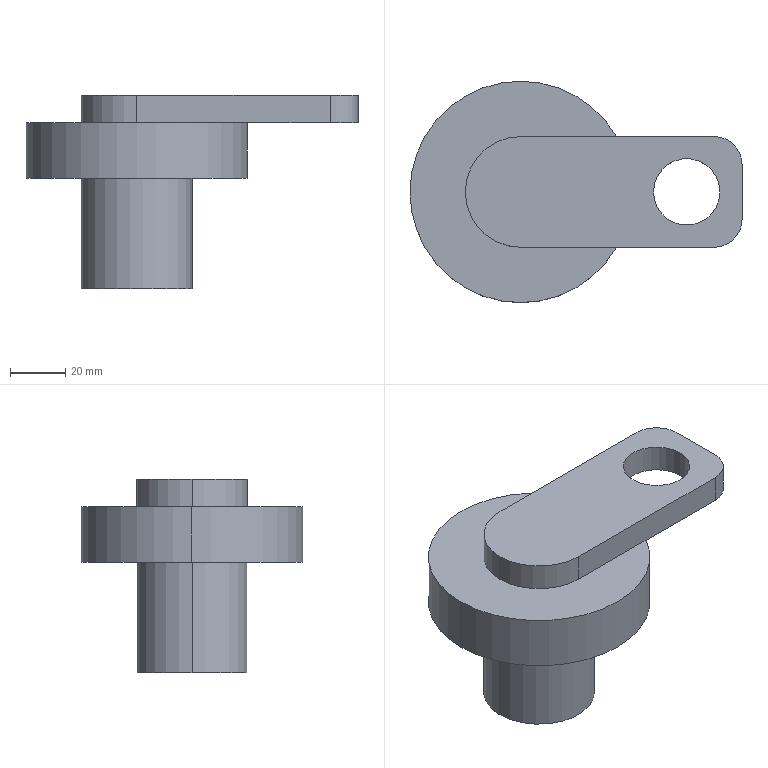Part | SolidWorks | features ICE 4, Extrusion 1, Fillet 1 | 1 solid | 18 faces | box 120 x 80 x 70 mm | volume 184127 mm3 | cylinder 10 | plane 8 | commonest cylinder face diameters 40 x4 20 x2 24 x2 80 x2
STEP:
#1=CARTESIAN_POINT('',(-10.,0.,-20.));
#2=VERTEX_POINT('',#1);
#3=CARTESIAN_POINT('',(-50.,0.,-20.));
#4=VERTEX_POINT('',#3);
#5=CARTESIAN_POINT('',(-30.,0.,-20.));
#6=DIRECTION('',(0.,0.,1.));
#7=DIRECTION('',(-1.,0.,0.));
#8=AXIS2_PLACEMENT_3D('',#5,#6,#7);
#9=CIRCLE('',#8,20.);
#10=EDGE_CURVE('',#2,#4,#9,.T.);
#11=ORIENTED_EDGE('',*,*,#10,.F.);
#12=CARTESIAN_POINT('',(-10.,0.,-60.));
#13=VERTEX_POINT('',#12);
#14=CARTESIAN_POINT('',(-10.,0.,10.));
#15=DIRECTION('',(0.,0.,-1.));
#16=VECTOR('',#15,1000.);
#17=LINE('',#14,#16);
#18=EDGE_CURVE('',#2,#13,#17,.T.);
#19=ORIENTED_EDGE('',*,*,#18,.T.);
#20=CARTESIAN_POINT('',(-50.,0.,-60.));
#21=VERTEX_POINT('',#20);
#22=CARTESIAN_POINT('',(-30.,0.,-60.));
#23=DIRECTION('',(0.,0.,-1.));
#24=DIRECTION('',(-1.,0.,0.));
#25=AXIS2_PLACEMENT_3D('',#22,#23,#24);
#26=CIRCLE('',#25,20.);
#27=EDGE_CURVE('',#21,#13,#26,.T.);
#28=ORIENTED_EDGE('',*,*,#27,.F.);
#29=CARTESIAN_POINT('',(-50.,0.,10.));
#30=DIRECTION('',(0.,0.,-1.));
#31=VECTOR('',#30,1000.);
#32=LINE('',#29,#31);
#33=EDGE_CURVE('',#4,#21,#32,.T.);
#34=ORIENTED_EDGE('',*,*,#33,.F.);
#35=EDGE_LOOP('',(#11,#19,#28,#34));
#36=FACE_OUTER_BOUND('',#35,.T.);
#37=CARTESIAN_POINT('',(-30.,0.,10.));
#38=DIRECTION('',(0.,0.,-1.));
#39=DIRECTION('',(-1.,0.,0.));
#40=AXIS2_PLACEMENT_3D('',#37,#38,#39);
#41=CYLINDRICAL_SURFACE('',#40,20.);
#42=ADVANCED_FACE('',(#36),#41,.T.);
#43=CARTESIAN_POINT('',(-70.,0.,-20.));
#44=VERTEX_POINT('',#43);
#45=CARTESIAN_POINT('',(10.,0.,-20.));
#46=VERTEX_POINT('',#45);
#47=CARTESIAN_POINT('',(-30.,0.,-20.));
#48=DIRECTION('',(0.,0.,-1.));
#49=DIRECTION('',(-1.,0.,0.));
#50=AXIS2_PLACEMENT_3D('',#47,#48,#49);
#51=CIRCLE('',#50,40.);
#52=EDGE_CURVE('',#44,#46,#51,.T.);
#53=ORIENTED_EDGE('',*,*,#52,.F.);
#54=CARTESIAN_POINT('',(-70.,0.,0.));
#55=VERTEX_POINT('',#54);
#56=CARTESIAN_POINT('',(-70.,0.,-20.));
#57=DIRECTION('',(0.,0.,1.));
#58=VECTOR('',#57,1000.);
#59=LINE('',#56,#58);
#60=EDGE_CURVE('',#44,#55,#59,.T.);
#61=ORIENTED_EDGE('',*,*,#60,.T.);
#62=CARTESIAN_POINT('',(4.641,20.,0.));
#63=VERTEX_POINT('',#62);
#64=CARTESIAN_POINT('',(-30.,0.,0.));
#65=DIRECTION('',(0.,0.,-1.));
#66=DIRECTION('',(-1.,0.,0.));
#67=AXIS2_PLACEMENT_3D('',#64,#65,#66);
#68=CIRCLE('',#67,40.);
#69=EDGE_CURVE('',#55,#63,#68,.T.);
#70=ORIENTED_EDGE('',*,*,#69,.T.);
#71=CARTESIAN_POINT('',(10.,0.,0.));
#72=VERTEX_POINT('',#71);
#73=CARTESIAN_POINT('',(-30.,0.,0.));
#74=DIRECTION('',(0.,0.,-1.));
#75=DIRECTION('',(-1.,0.,0.));
#76=AXIS2_PLACEMENT_3D('',#73,#74,#75);
#77=CIRCLE('',#76,40.);
#78=EDGE_CURVE('',#63,#72,#77,.T.);
#79=ORIENTED_EDGE('',*,*,#78,.T.);
#80=CARTESIAN_POINT('',(10.,0.,-20.));
#81=DIRECTION('',(0.,0.,1.));
#82=VECTOR('',#81,1000.);
#83=LINE('',#80,#82);
#84=EDGE_CURVE('',#46,#72,#83,.T.);
#85=ORIENTED_EDGE('',*,*,#84,.F.);
#86=EDGE_LOOP('',(#53,#61,#70,#79,#85));
#87=FACE_OUTER_BOUND('',#86,.T.);
#88=CARTESIAN_POINT('',(-30.,0.,-20.));
#89=DIRECTION('',(0.,0.,1.));
#90=DIRECTION('',(1.,0.,0.));
#91=AXIS2_PLACEMENT_3D('',#88,#89,#90);
#92=CYLINDRICAL_SURFACE('',#91,40.);
#93=ADVANCED_FACE('',(#87),#92,.T.);
#94=CARTESIAN_POINT('',(18.,0.,0.));
#95=VERTEX_POINT('',#94);
#96=CARTESIAN_POINT('',(42.,0.,0.));
#97=VERTEX_POINT('',#96);
#98=CARTESIAN_POINT('',(30.,0.,0.));
#99=DIRECTION('',(0.,0.,1.));
#100=DIRECTION('',(1.,0.,0.));
#101=AXIS2_PLACEMENT_3D('',#98,#99,#100);
#102=CIRCLE('',#101,12.);
#103=EDGE_CURVE('',#95,#97,#102,.T.);
#104=ORIENTED_EDGE('',*,*,#103,.F.);
#105=CARTESIAN_POINT('',(18.,0.,10.));
#106=VERTEX_POINT('',#105);
#107=CARTESIAN_POINT('',(18.,0.,0.));
#108=DIRECTION('',(0.,0.,1.));
#109=VECTOR('',#108,1000.);
#110=LINE('',#107,#109);
#111=EDGE_CURVE('',#95,#106,#110,.T.);
#112=ORIENTED_EDGE('',*,*,#111,.T.);
#113=CARTESIAN_POINT('',(42.,0.,10.));
#114=VERTEX_POINT('',#113);
#115=CARTESIAN_POINT('',(30.,0.,10.));
#116=DIRECTION('',(0.,0.,1.));
#117=DIRECTION('',(1.,0.,0.));
#118=AXIS2_PLACEMENT_3D('',#115,#116,#117);
#119=CIRCLE('',#118,12.);
#120=EDGE_CURVE('',#106,#114,#119,.T.);
#121=ORIENTED_EDGE('',*,*,#120,.T.);
#122=CARTESIAN_POINT('',(42.,0.,0.));
#123=DIRECTION('',(0.,0.,1.));
#124=VECTOR('',#123,1000.);
#125=LINE('',#122,#124);
#126=EDGE_CURVE('',#97,#114,#125,.T.);
#127=ORIENTED_EDGE('',*,*,#126,.F.);
#128=EDGE_LOOP('',(#104,#112,#121,#127));
#129=FACE_OUTER_BOUND('',#128,.T.);
#130=CARTESIAN_POINT('',(30.,0.,0.));
#131=DIRECTION('',(0.,0.,1.));
#132=DIRECTION('',(1.,0.,0.));
#133=AXIS2_PLACEMENT_3D('',#130,#131,#132);
#134=CYLINDRICAL_SURFACE('',#133,12.);
#135=ADVANCED_FACE('',(#129),#134,.F.);
#136=CARTESIAN_POINT('',(-30.,-20.,10.));
#137=VERTEX_POINT('',#136);
#138=CARTESIAN_POINT('',(-50.,0.,10.));
#139=VERTEX_POINT('',#138);
#140=CARTESIAN_POINT('',(-30.,0.,10.));
#141=DIRECTION('',(0.,0.,-1.));
#142=DIRECTION('',(-1.,0.,0.));
#143=AXIS2_PLACEMENT_3D('',#140,#141,#142);
#144=CIRCLE('',#143,20.);
#145=EDGE_CURVE('',#137,#139,#144,.T.);
#146=ORIENTED_EDGE('',*,*,#145,.T.);
#147=CARTESIAN_POINT('',(-50.,0.,0.));
#148=VERTEX_POINT('',#147);
#149=CARTESIAN_POINT('',(-50.,0.,10.));
#150=DIRECTION('',(0.,0.,-1.));
#151=VECTOR('',#150,1000.);
#152=LINE('',#149,#151);
#153=EDGE_CURVE('',#139,#148,#152,.T.);
#154=ORIENTED_EDGE('',*,*,#153,.T.);
#155=CARTESIAN_POINT('',(-30.,-20.,0.));
#156=VERTEX_POINT('',#155);
#157=CARTESIAN_POINT('',(-30.,0.,0.));
#158=DIRECTION('',(0.,0.,1.));
#159=DIRECTION('',(-1.,0.,0.));
#160=AXIS2_PLACEMENT_3D('',#157,#158,#159);
#161=CIRCLE('',#160,20.);
#162=EDGE_CURVE('',#148,#156,#161,.T.);
#163=ORIENTED_EDGE('',*,*,#162,.T.);
#164=CARTESIAN_POINT('',(-30.,-20.,10.));
#165=DIRECTION('',(0.,0.,-1.));
#166=VECTOR('',#165,1000.);
#167=LINE('',#164,#166);
#168=EDGE_CURVE('',#137,#156,#167,.T.);
#169=ORIENTED_EDGE('',*,*,#168,.F.);
#170=EDGE_LOOP('',(#146,#154,#163,#169));
#171=FACE_OUTER_BOUND('',#170,.T.);
#172=CARTESIAN_POINT('',(-30.,0.,10.));
#173=DIRECTION('',(0.,0.,-1.));
#174=DIRECTION('',(-1.,0.,0.));
#175=AXIS2_PLACEMENT_3D('',#172,#173,#174);
#176=CYLINDRICAL_SURFACE('',#175,20.);
#177=ADVANCED_FACE('',(#171),#176,.T.);
#178=ORIENTED_EDGE('',*,*,#153,.F.);
#179=CARTESIAN_POINT('',(-30.,20.,10.));
#180=VERTEX_POINT('',#179);
#181=CARTESIAN_POINT('',(-30.,0.,10.));
#182=DIRECTION('',(0.,0.,-1.));
#183=DIRECTION('',(-1.,0.,0.));
#184=AXIS2_PLACEMENT_3D('',#181,#182,#183);
#185=CIRCLE('',#184,20.);
#186=EDGE_CURVE('',#139,#180,#185,.T.);
#187=ORIENTED_EDGE('',*,*,#186,.T.);
#188=CARTESIAN_POINT('',(-30.,20.,0.));
#189=VERTEX_POINT('',#188);
#190=CARTESIAN_POINT('',(-30.,20.,10.));
#191=DIRECTION('',(0.,0.,-1.));
#192=VECTOR('',#191,1000.);
#193=LINE('',#190,#192);
#194=EDGE_CURVE('',#180,#189,#193,.T.);
#195=ORIENTED_EDGE('',*,*,#194,.T.);
#196=CARTESIAN_POINT('',(-30.,0.,0.));
#197=DIRECTION('',(0.,0.,1.));
#198=DIRECTION('',(-1.,0.,0.));
#199=AXIS2_PLACEMENT_3D('',#196,#197,#198);
#200=CIRCLE('',#199,20.);
#201=EDGE_CURVE('',#189,#148,#200,.T.);
#202=ORIENTED_EDGE('',*,*,#201,.T.);
#203=EDGE_LOOP('',(#178,#187,#195,#202));
#204=FACE_OUTER_BOUND('',#203,.T.);
#205=CARTESIAN_POINT('',(-30.,0.,10.));
#206=DIRECTION('',(0.,0.,-1.));
#207=DIRECTION('',(-1.,0.,0.));
#208=AXIS2_PLACEMENT_3D('',#205,#206,#207);
#209=CYLINDRICAL_SURFACE('',#208,20.);
#210=ADVANCED_FACE('',(#204),#209,.T.);
#211=ORIENTED_EDGE('',*,*,#78,.F.);
#212=CARTESIAN_POINT('',(40.,20.,0.));
#213=VERTEX_POINT('',#212);
#214=CARTESIAN_POINT('',(-50.,20.,0.));
#215=DIRECTION('',(-1.,0.,0.));
#216=VECTOR('',#215,1000.);
#217=LINE('',#214,#216);
#218=EDGE_CURVE('',#213,#63,#217,.T.);
#219=ORIENTED_EDGE('',*,*,#218,.F.);
#220=CARTESIAN_POINT('',(50.,10.,0.));
#221=VERTEX_POINT('',#220);
#222=CARTESIAN_POINT('',(40.,10.,0.));
#223=DIRECTION('',(0.,0.,-1.));
#224=DIRECTION('',(1.,0.,0.));
#225=AXIS2_PLACEMENT_3D('',#222,#223,#224);
#226=CIRCLE('',#225,10.);
#227=EDGE_CURVE('',#213,#221,#226,.T.);
#228=ORIENTED_EDGE('',*,*,#227,.T.);
#229=CARTESIAN_POINT('',(50.,-10.,0.));
#230=VERTEX_POINT('',#229);
#231=CARTESIAN_POINT('',(50.,20.,0.));
#232=DIRECTION('',(0.,1.,0.));
#233=VECTOR('',#232,1000.);
#234=LINE('',#231,#233);
#235=EDGE_CURVE('',#230,#221,#234,.T.);
#236=ORIENTED_EDGE('',*,*,#235,.F.);
#237=CARTESIAN_POINT('',(40.,-20.,0.));
#238=VERTEX_POINT('',#237);
#239=CARTESIAN_POINT('',(40.,-10.,0.));
#240=DIRECTION('',(0.,0.,-1.));
#241=DIRECTION('',(1.,0.,0.));
#242=AXIS2_PLACEMENT_3D('',#239,#240,#241);
#243=CIRCLE('',#242,10.);
#244=EDGE_CURVE('',#230,#238,#243,.T.);
#245=ORIENTED_EDGE('',*,*,#244,.T.);
#246=CARTESIAN_POINT('',(4.641,-20.,0.));
#247=VERTEX_POINT('',#246);
#248=CARTESIAN_POINT('',(-50.,-20.,0.));
#249=DIRECTION('',(1.,0.,0.));
#250=VECTOR('',#249,1000.);
#251=LINE('',#248,#250);
#252=EDGE_CURVE('',#247,#238,#251,.T.);
#253=ORIENTED_EDGE('',*,*,#252,.F.);
#254=CARTESIAN_POINT('',(-30.,0.,0.));
#255=DIRECTION('',(0.,0.,-1.));
#256=DIRECTION('',(-1.,0.,0.));
#257=AXIS2_PLACEMENT_3D('',#254,#255,#256);
#258=CIRCLE('',#257,40.);
#259=EDGE_CURVE('',#72,#247,#258,.T.);
#260=ORIENTED_EDGE('',*,*,#259,.F.);
#261=EDGE_LOOP('',(#211,#219,#228,#236,#245,#253,#260));
#262=FACE_OUTER_BOUND('',#261,.T.);
#263=CARTESIAN_POINT('',(30.,0.,0.));
#264=DIRECTION('',(0.,0.,1.));
#265=DIRECTION('',(1.,0.,0.));
#266=AXIS2_PLACEMENT_3D('',#263,#264,#265);
#267=CIRCLE('',#266,12.);
#268=EDGE_CURVE('',#97,#95,#267,.T.);
#269=ORIENTED_EDGE('',*,*,#268,.T.);
#270=ORIENTED_EDGE('',*,*,#103,.T.);
#271=EDGE_LOOP('',(#269,#270));
#272=FACE_BOUND('',#271,.T.);
#273=CARTESIAN_POINT('',(0.,0.,0.));
#274=DIRECTION('',(0.,0.,1.));
#275=DIRECTION('',(1.,0.,0.));
#276=AXIS2_PLACEMENT_3D('',#273,#274,#275);
#277=PLANE('',#276);
#278=ADVANCED_FACE('',(#262,#272),#277,.F.);
#279=CARTESIAN_POINT('',(30.,0.,10.));
#280=DIRECTION('',(0.,0.,1.));
#281=DIRECTION('',(1.,0.,0.));
#282=AXIS2_PLACEMENT_3D('',#279,#280,#281);
#283=CIRCLE('',#282,12.);
#284=EDGE_CURVE('',#114,#106,#283,.T.);
#285=ORIENTED_EDGE('',*,*,#284,.F.);
#286=ORIENTED_EDGE('',*,*,#120,.F.);
#287=EDGE_LOOP('',(#285,#286));
#288=FACE_BOUND('',#287,.T.);
#289=ORIENTED_EDGE('',*,*,#145,.F.);
#290=CARTESIAN_POINT('',(40.,-20.,10.));
#291=VERTEX_POINT('',#290);
#292=CARTESIAN_POINT('',(-50.,-20.,10.));
#293=DIRECTION('',(1.,0.,0.));
#294=VECTOR('',#293,1000.);
#295=LINE('',#292,#294);
#296=EDGE_CURVE('',#137,#291,#295,.T.);
#297=ORIENTED_EDGE('',*,*,#296,.T.);
#298=CARTESIAN_POINT('',(50.,-10.,10.));
#299=VERTEX_POINT('',#298);
#300=CARTESIAN_POINT('',(40.,-10.,10.));
#301=DIRECTION('',(0.,0.,1.));
#302=DIRECTION('',(1.,0.,0.));
#303=AXIS2_PLACEMENT_3D('',#300,#301,#302);
#304=CIRCLE('',#303,10.);
#305=EDGE_CURVE('',#291,#299,#304,.T.);
#306=ORIENTED_EDGE('',*,*,#305,.T.);
#307=CARTESIAN_POINT('',(50.,10.,10.));
#308=VERTEX_POINT('',#307);
#309=CARTESIAN_POINT('',(50.,20.,10.));
#310=DIRECTION('',(0.,1.,0.));
#311=VECTOR('',#310,1000.);
#312=LINE('',#309,#311);
#313=EDGE_CURVE('',#299,#308,#312,.T.);
#314=ORIENTED_EDGE('',*,*,#313,.T.);
#315=CARTESIAN_POINT('',(40.,20.,10.));
#316=VERTEX_POINT('',#315);
#317=CARTESIAN_POINT('',(40.,10.,10.));
#318=DIRECTION('',(0.,0.,1.));
#319=DIRECTION('',(1.,0.,0.));
#320=AXIS2_PLACEMENT_3D('',#317,#318,#319);
#321=CIRCLE('',#320,10.);
#322=EDGE_CURVE('',#308,#316,#321,.T.);
#323=ORIENTED_EDGE('',*,*,#322,.T.);
#324=CARTESIAN_POINT('',(-50.,20.,10.));
#325=DIRECTION('',(-1.,0.,0.));
#326=VECTOR('',#325,1000.);
#327=LINE('',#324,#326);
#328=EDGE_CURVE('',#316,#180,#327,.T.);
#329=ORIENTED_EDGE('',*,*,#328,.T.);
#330=ORIENTED_EDGE('',*,*,#186,.F.);
#331=EDGE_LOOP('',(#289,#297,#306,#314,#323,#329,#330));
#332=FACE_OUTER_BOUND('',#331,.T.);
#333=CARTESIAN_POINT('',(0.,0.,10.));
#334=DIRECTION('',(0.,0.,1.));
#335=DIRECTION('',(1.,0.,0.));
#336=AXIS2_PLACEMENT_3D('',#333,#334,#335);
#337=PLANE('',#336);
#338=ADVANCED_FACE('',(#288,#332),#337,.T.);
#339=ORIENTED_EDGE('',*,*,#194,.F.);
#340=ORIENTED_EDGE('',*,*,#328,.F.);
#341=CARTESIAN_POINT('',(40.,20.,10.));
#342=DIRECTION('',(0.,0.,-1.));
#343=VECTOR('',#342,1000.);
#344=LINE('',#341,#343);
#345=EDGE_CURVE('',#316,#213,#344,.T.);
#346=ORIENTED_EDGE('',*,*,#345,.T.);
#347=ORIENTED_EDGE('',*,*,#218,.T.);
#348=CARTESIAN_POINT('',(-50.,20.,0.));
#349=DIRECTION('',(1.,0.,0.));
#350=VECTOR('',#349,1000.);
#351=LINE('',#348,#350);
#352=EDGE_CURVE('',#189,#63,#351,.T.);
#353=ORIENTED_EDGE('',*,*,#352,.F.);
#354=EDGE_LOOP('',(#339,#340,#346,#347,#353));
#355=FACE_OUTER_BOUND('',#354,.T.);
#356=CARTESIAN_POINT('',(-50.,20.,10.));
#357=DIRECTION('',(0.,-1.,0.));
#358=DIRECTION('',(0.,0.,-1.));
#359=AXIS2_PLACEMENT_3D('',#356,#357,#358);
#360=PLANE('',#359);
#361=ADVANCED_FACE('',(#355),#360,.F.);
#362=ORIENTED_EDGE('',*,*,#313,.F.);
#363=CARTESIAN_POINT('',(50.,-10.,10.));
#364=DIRECTION('',(0.,0.,-1.));
#365=VECTOR('',#364,1000.);
#366=LINE('',#363,#365);
#367=EDGE_CURVE('',#299,#230,#366,.T.);
#368=ORIENTED_EDGE('',*,*,#367,.T.);
#369=ORIENTED_EDGE('',*,*,#235,.T.);
#370=CARTESIAN_POINT('',(50.,10.,10.));
#371=DIRECTION('',(0.,0.,1.));
#372=VECTOR('',#371,1000.);
#373=LINE('',#370,#372);
#374=EDGE_CURVE('',#221,#308,#373,.T.);
#375=ORIENTED_EDGE('',*,*,#374,.T.);
#376=EDGE_LOOP('',(#362,#368,#369,#375));
#377=FACE_OUTER_BOUND('',#376,.T.);
#378=CARTESIAN_POINT('',(50.,20.,10.));
#379=DIRECTION('',(-1.,0.,0.));
#380=DIRECTION('',(0.,-1.,0.));
#381=AXIS2_PLACEMENT_3D('',#378,#379,#380);
#382=PLANE('',#381);
#383=ADVANCED_FACE('',(#377),#382,.F.);
#384=ORIENTED_EDGE('',*,*,#296,.F.);
#385=ORIENTED_EDGE('',*,*,#168,.T.);
#386=CARTESIAN_POINT('',(-50.,-20.,0.));
#387=DIRECTION('',(1.,0.,0.));
#388=VECTOR('',#387,1000.);
#389=LINE('',#386,#388);
#390=EDGE_CURVE('',#156,#247,#389,.T.);
#391=ORIENTED_EDGE('',*,*,#390,.T.);
#392=ORIENTED_EDGE('',*,*,#252,.T.);
#393=CARTESIAN_POINT('',(40.,-20.,10.));
#394=DIRECTION('',(0.,0.,1.));
#395=VECTOR('',#394,1000.);
#396=LINE('',#393,#395);
#397=EDGE_CURVE('',#238,#291,#396,.T.);
#398=ORIENTED_EDGE('',*,*,#397,.T.);
#399=EDGE_LOOP('',(#384,#385,#391,#392,#398));
#400=FACE_OUTER_BOUND('',#399,.T.);
#401=CARTESIAN_POINT('',(-50.,-20.,10.));
#402=DIRECTION('',(0.,1.,0.));
#403=DIRECTION('',(0.,0.,1.));
#404=AXIS2_PLACEMENT_3D('',#401,#402,#403);
#405=PLANE('',#404);
#406=ADVANCED_FACE('',(#400),#405,.F.);
#407=ORIENTED_EDGE('',*,*,#111,.F.);
#408=ORIENTED_EDGE('',*,*,#268,.F.);
#409=ORIENTED_EDGE('',*,*,#126,.T.);
#410=ORIENTED_EDGE('',*,*,#284,.T.);
#411=EDGE_LOOP('',(#407,#408,#409,#410));
#412=FACE_OUTER_BOUND('',#411,.T.);
#413=CARTESIAN_POINT('',(30.,0.,0.));
#414=DIRECTION('',(0.,0.,1.));
#415=DIRECTION('',(1.,0.,0.));
#416=AXIS2_PLACEMENT_3D('',#413,#414,#415);
#417=CYLINDRICAL_SURFACE('',#416,12.);
#418=ADVANCED_FACE('',(#412),#417,.F.);
#419=ORIENTED_EDGE('',*,*,#305,.F.);
#420=ORIENTED_EDGE('',*,*,#397,.F.);
#421=ORIENTED_EDGE('',*,*,#244,.F.);
#422=ORIENTED_EDGE('',*,*,#367,.F.);
#423=EDGE_LOOP('',(#419,#420,#421,#422));
#424=FACE_OUTER_BOUND('',#423,.T.);
#425=CARTESIAN_POINT('',(40.,-10.,10.));
#426=DIRECTION('',(0.,0.,-1.));
#427=DIRECTION('',(-1.,0.,0.));
#428=AXIS2_PLACEMENT_3D('',#425,#426,#427);
#429=CYLINDRICAL_SURFACE('',#428,10.);
#430=ADVANCED_FACE('',(#424),#429,.T.);
#431=ORIENTED_EDGE('',*,*,#322,.F.);
#432=ORIENTED_EDGE('',*,*,#374,.F.);
#433=ORIENTED_EDGE('',*,*,#227,.F.);
#434=ORIENTED_EDGE('',*,*,#345,.F.);
#435=EDGE_LOOP('',(#431,#432,#433,#434));
#436=FACE_OUTER_BOUND('',#435,.T.);
#437=CARTESIAN_POINT('',(40.,10.,10.));
#438=DIRECTION('',(0.,0.,-1.));
#439=DIRECTION('',(-1.,0.,0.));
#440=AXIS2_PLACEMENT_3D('',#437,#438,#439);
#441=CYLINDRICAL_SURFACE('',#440,10.);
#442=ADVANCED_FACE('',(#436),#441,.T.);
#443=ORIENTED_EDGE('',*,*,#201,.F.);
#444=ORIENTED_EDGE('',*,*,#352,.T.);
#445=ORIENTED_EDGE('',*,*,#69,.F.);
#446=CARTESIAN_POINT('',(-30.,0.,0.));
#447=DIRECTION('',(0.,0.,-1.));
#448=DIRECTION('',(-1.,0.,0.));
#449=AXIS2_PLACEMENT_3D('',#446,#447,#448);
#450=CIRCLE('',#449,40.);
#451=EDGE_CURVE('',#247,#55,#450,.T.);
#452=ORIENTED_EDGE('',*,*,#451,.F.);
#453=ORIENTED_EDGE('',*,*,#390,.F.);
#454=ORIENTED_EDGE('',*,*,#162,.F.);
#455=EDGE_LOOP('',(#443,#444,#445,#452,#453,#454));
#456=FACE_OUTER_BOUND('',#455,.T.);
#457=CARTESIAN_POINT('',(-30.,0.,0.));
#458=DIRECTION('',(0.,0.,-1.));
#459=DIRECTION('',(-1.,0.,0.));
#460=AXIS2_PLACEMENT_3D('',#457,#458,#459);
#461=PLANE('',#460);
#462=ADVANCED_FACE('',(#456),#461,.F.);
#463=ORIENTED_EDGE('',*,*,#60,.F.);
#464=CARTESIAN_POINT('',(-30.,0.,-20.));
#465=DIRECTION('',(0.,0.,-1.));
#466=DIRECTION('',(-1.,0.,0.));
#467=AXIS2_PLACEMENT_3D('',#464,#465,#466);
#468=CIRCLE('',#467,40.);
#469=EDGE_CURVE('',#46,#44,#468,.T.);
#470=ORIENTED_EDGE('',*,*,#469,.F.);
#471=ORIENTED_EDGE('',*,*,#84,.T.);
#472=ORIENTED_EDGE('',*,*,#259,.T.);
#473=ORIENTED_EDGE('',*,*,#451,.T.);
#474=EDGE_LOOP('',(#463,#470,#471,#472,#473));
#475=FACE_OUTER_BOUND('',#474,.T.);
#476=CARTESIAN_POINT('',(-30.,0.,-20.));
#477=DIRECTION('',(0.,0.,1.));
#478=DIRECTION('',(1.,0.,0.));
#479=AXIS2_PLACEMENT_3D('',#476,#477,#478);
#480=CYLINDRICAL_SURFACE('',#479,40.);
#481=ADVANCED_FACE('',(#475),#480,.T.);
#482=CARTESIAN_POINT('',(-30.,0.,-20.));
#483=DIRECTION('',(0.,0.,1.));
#484=DIRECTION('',(-1.,0.,0.));
#485=AXIS2_PLACEMENT_3D('',#482,#483,#484);
#486=CIRCLE('',#485,20.);
#487=EDGE_CURVE('',#4,#2,#486,.T.);
#488=ORIENTED_EDGE('',*,*,#487,.T.);
#489=ORIENTED_EDGE('',*,*,#10,.T.);
#490=EDGE_LOOP('',(#488,#489));
#491=FACE_BOUND('',#490,.T.);
#492=ORIENTED_EDGE('',*,*,#469,.T.);
#493=ORIENTED_EDGE('',*,*,#52,.T.);
#494=EDGE_LOOP('',(#492,#493));
#495=FACE_OUTER_BOUND('',#494,.T.);
#496=CARTESIAN_POINT('',(-30.,0.,-20.));
#497=DIRECTION('',(0.,0.,-1.));
#498=DIRECTION('',(-1.,0.,0.));
#499=AXIS2_PLACEMENT_3D('',#496,#497,#498);
#500=PLANE('',#499);
#501=ADVANCED_FACE('',(#491,#495),#500,.T.);
#502=ORIENTED_EDGE('',*,*,#27,.T.);
#503=CARTESIAN_POINT('',(-30.,0.,-60.));
#504=DIRECTION('',(0.,0.,-1.));
#505=DIRECTION('',(-1.,0.,0.));
#506=AXIS2_PLACEMENT_3D('',#503,#504,#505);
#507=CIRCLE('',#506,20.);
#508=EDGE_CURVE('',#13,#21,#507,.T.);
#509=ORIENTED_EDGE('',*,*,#508,.T.);
#510=EDGE_LOOP('',(#502,#509));
#511=FACE_OUTER_BOUND('',#510,.T.);
#512=CARTESIAN_POINT('',(-30.,0.,-60.));
#513=DIRECTION('',(0.,0.,-1.));
#514=DIRECTION('',(-1.,0.,0.));
#515=AXIS2_PLACEMENT_3D('',#512,#513,#514);
#516=PLANE('',#515);
#517=ADVANCED_FACE('',(#511),#516,.T.);
#518=ORIENTED_EDGE('',*,*,#18,.F.);
#519=ORIENTED_EDGE('',*,*,#487,.F.);
#520=ORIENTED_EDGE('',*,*,#33,.T.);
#521=ORIENTED_EDGE('',*,*,#508,.F.);
#522=EDGE_LOOP('',(#518,#519,#520,#521));
#523=FACE_OUTER_BOUND('',#522,.T.);
#524=CARTESIAN_POINT('',(-30.,0.,10.));
#525=DIRECTION('',(0.,0.,-1.));
#526=DIRECTION('',(-1.,0.,0.));
#527=AXIS2_PLACEMENT_3D('',#524,#525,#526);
#528=CYLINDRICAL_SURFACE('',#527,20.);
#529=ADVANCED_FACE('',(#523),#528,.T.);
#530=CLOSED_SHELL('',(#42,#93,#135,#177,#210,#278,#338,#361,#383,#406,#418,#430,#442,#462,#481,#501,#517,#529));
#531=MANIFOLD_SOLID_BREP('',#530);
#532=CARTESIAN_POINT('',(0.,0.,0.));
#533=DIRECTION('',(0.,0.,1.));
#534=DIRECTION('',(1.,0.,0.));
#535=AXIS2_PLACEMENT_3D('',#532,#533,#534);
#536=(LENGTH_UNIT()NAMED_UNIT(*)SI_UNIT(.MILLI.,.METRE.));
#537=UNCERTAINTY_MEASURE_WITH_UNIT(LENGTH_MEASURE(0.00001),#536,'','');
#538=(NAMED_UNIT(*)PLANE_ANGLE_UNIT()SI_UNIT($,.RADIAN.));
#539=(NAMED_UNIT(*)SI_UNIT($,.STERADIAN.)SOLID_ANGLE_UNIT());
#540=(GEOMETRIC_REPRESENTATION_CONTEXT(3)GLOBAL_UNCERTAINTY_ASSIGNED_CONTEXT((#537))GLOBAL_UNIT_ASSIGNED_CONTEXT((#536,#538,#539))REPRESENTATION_CONTEXT('',''));
#541=ADVANCED_BREP_SHAPE_REPRESENTATION('',(#531,#535),#540);